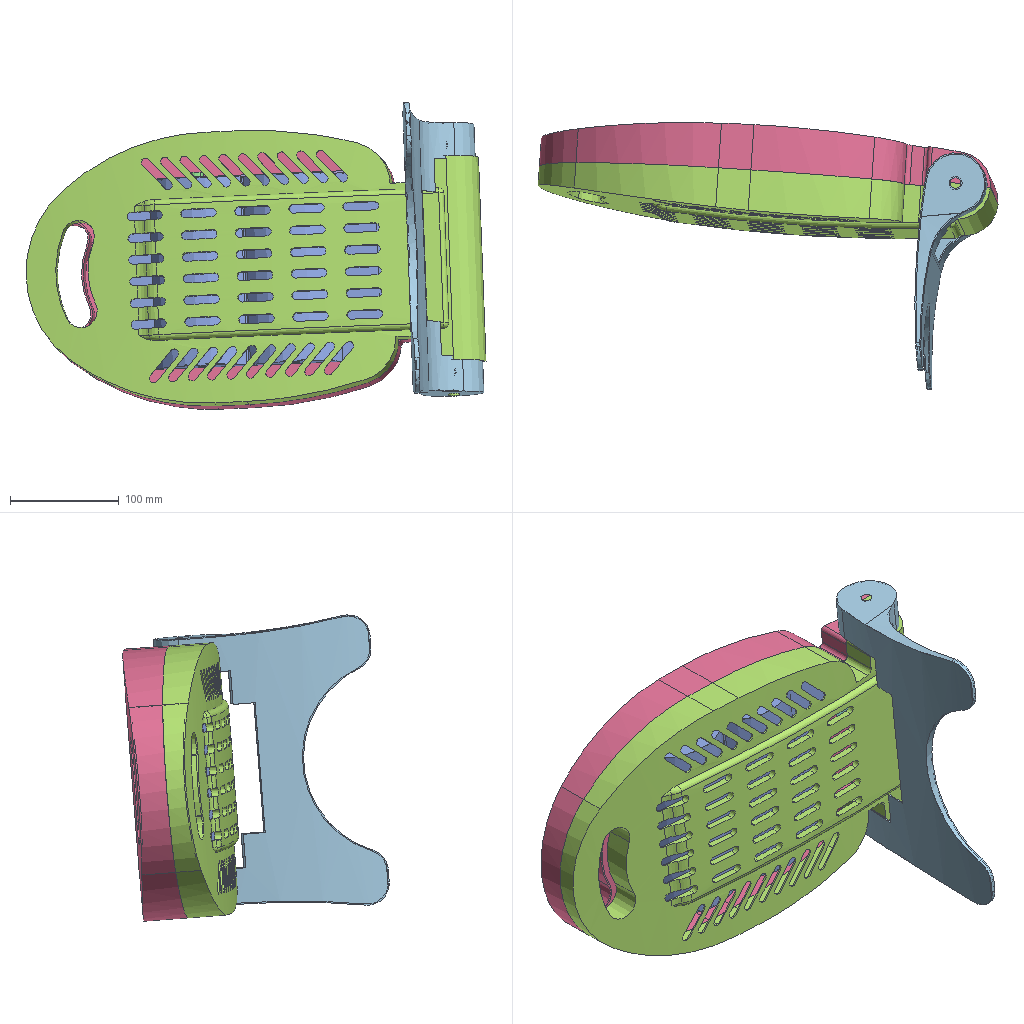Assembly | SolidWorks | 11 different items | 12 placed | box 424 x 245 x 282 mm
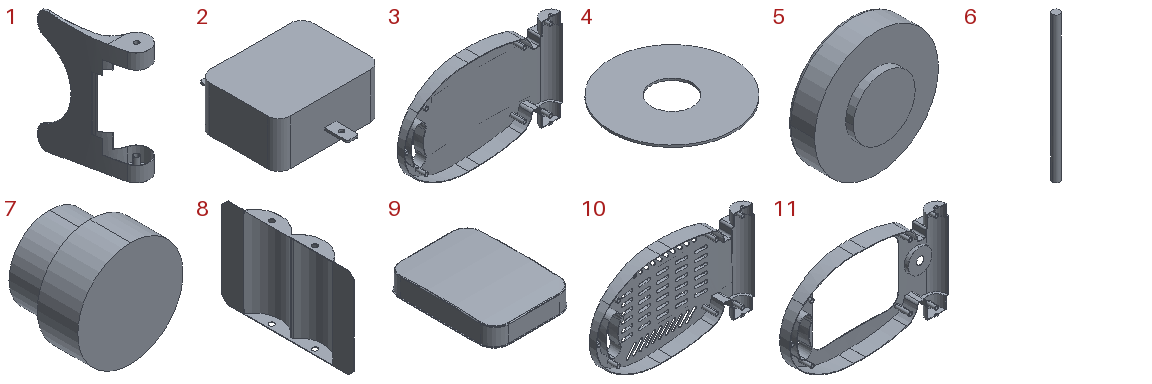Parts list (item | quantity | size | volume | features):
1 | x1 | 77.001 x 196 x 268.141 mm | 67561 mm3 | features ICE 3, Extrusion 1, Shell 1
2 | x1 | 45 x 55 x 20 mm | 31190 mm3 | features ICE 2, Extrusion 1
3 | x1 | 420 x 43.06 x 250 mm | 378076 mm3 | features ICE 7, Fillet 2, CombineBodies 1, Extrusion 1, Shell 1
4 | x1 | 60 x 60 x 1 mm | 2513 mm3 | features Extrusion 1
5 | x1 | 40 x 15 x 40 mm | 12868 mm3 | features ICE 3, Fillet 1, RevCut 1, Revolution 1
6 | x2 | 9 x 9 x 174 mm | 11069 mm3 | features Extrusion 1
7 | x1 | 13 x 10 x 13 mm | 805.033 mm3 | features Revolution 1
8 | x1 | 27.127 x 256 x 174 mm | 56067 mm3 | features Chamfer 2, Extrusion 1, ICE 1, Shell 1
9 | x1 | 174 x 234 x 41.94 mm | 67886 mm3 | features ICE 2, Extrusion 1, Fillet 1, Shell 1
10 | x1 | 420 x 43.06 x 250 mm | 321322 mm3 | features ICE 8, Fillet 3, CombineBodies 1, Extrusion 1, MirrorPattern 1, Shell 1
11 | x1 | 420 x 41.94 x 250 mm | 152535 mm3 | features ICE 9, CombineBodies 1, Extrusion 1, Fillet 1, Shell 1
Mates (type | each side: item.copy, entity, surface, feature):
Concentric | 6.1 face cylinder Boss-Extrude1 | 8.1 face cylinder Cut-Extrude1
Concentric | 8.1 face cylinder Cut-Extrude1 | 6.2 face cylinder Boss-Extrude1
Coincident | 6.1 face plane Boss-Extrude1 | 8.1 face plane Boss-Extrude2
Coincident | 8.1 face plane Boss-Extrude2 | 6.2 face plane Boss-Extrude1
Concentric | 6.1 face cylinder Boss-Extrude1 | 7.1 face cylinder Revolve1
Coincident | 8.1 face plane Boss-Extrude2 | 7.1 face plane Revolve1
Concentric | 5.1 face cylinder Boss-Extrude1 | 4.1 face cylinder Boss-Extrude1
Coincident | 8.1 face plane Boss-Extrude2 | 9.1 face plane Boss-Extrude1 | 3 times
Coincident | 8.1 face plane Boss-Extrude2 | 2.1 face plane Boss-Extrude1 | 2 times
Concentric | 10.1 face cylinder Boss-Extrude3 | 11.1 face cylinder Boss-Extrude3
Coincident | 10.1 face plane Combine1 | 11.1 face plane Combine1
Coincident | 10.1 face plane Boss-Extrude4 | 11.1 face plane Boss-Extrude4
Concentric | 10.1 face cylinder Boss-Extrude3 | 1.1 face cylinder Shell1
Coincident | 11.1 face plane Boss-Extrude4 | 1.1 face plane Cut-Extrude5
Coincident | 5.1 face plane Revolve1 | 4.1 face plane Boss-Extrude1
Concentric | 5.1 face cylinder Boss-Extrude1 | 11.1 face cylinder Cut-Extrude9
Coincident | 4.1 face plane Boss-Extrude1 | 11.1 face plane Cut-Extrude7
Tangent | 10.1 face cylinder Boss-Extrude7 | 1.1 face plane Cut-Extrude8